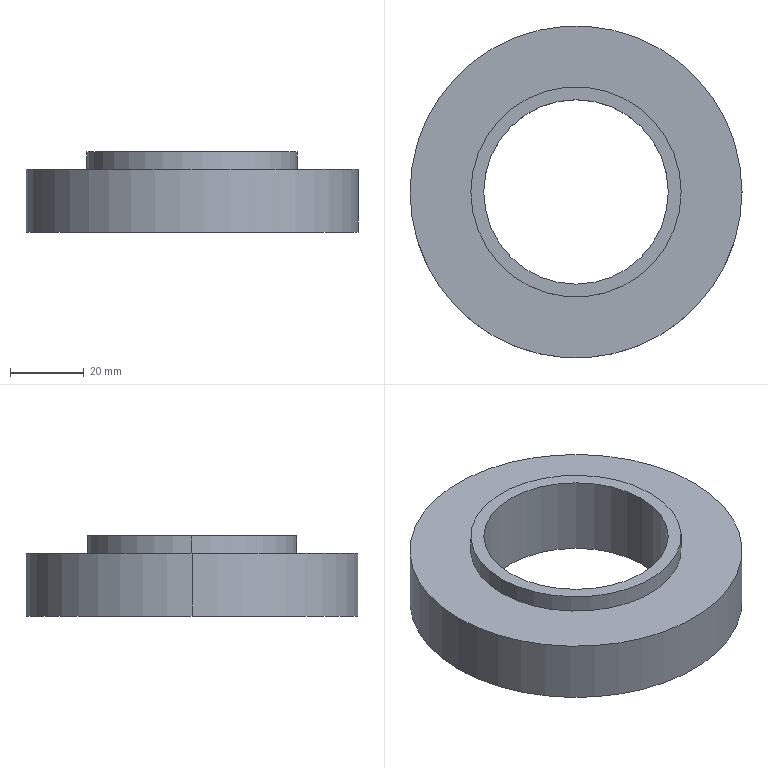Part | STEP file | 30210 | 1 solid | 9 faces | box 90 x 90 x 21.75 mm | volume 77564 mm3 | cylinder 6 | plane 3 | commonest cylinder face diameters 50 x2 57 x2 90 x2
STEP:
#1=CARTESIAN_POINT('',(0.,0.,0.));
#2=DIRECTION('',(0.,0.,1.));
#3=DIRECTION('',(1.,0.,0.));
#4=AXIS2_PLACEMENT_3D('',#1,#2,#3);
#5=CARTESIAN_POINT('',(-25.,0.,21.75));
#6=VERTEX_POINT('',#5);
#7=CARTESIAN_POINT('',(-25.,0.,0.));
#8=VERTEX_POINT('',#7);
#9=CARTESIAN_POINT('',(-25.,0.,21.75));
#10=DIRECTION('',(0.,0.,-1.));
#11=VECTOR('',#10,1.);
#12=LINE('',#9,#11);
#13=CARTESIAN_POINT('',(0.,0.,21.75));
#14=DIRECTION('',(0.,0.,-1.));
#15=DIRECTION('',(-1.,0.,0.));
#16=AXIS2_PLACEMENT_3D('',#13,#14,#15);
#17=CYLINDRICAL_SURFACE('',#16,25.);
#18=CARTESIAN_POINT('',(6.283,0.));
#19=DIRECTION('',(0.,1.));
#20=VECTOR('',#19,1.);
#21=LINE('',#18,#20);
#22=(GEOMETRIC_REPRESENTATION_CONTEXT(2)PARAMETRIC_REPRESENTATION_CONTEXT()REPRESENTATION_CONTEXT('',''));
#23=DEFINITIONAL_REPRESENTATION('',(#21),#22);
#24=PCURVE('',#17,#23);
#25=CARTESIAN_POINT('',(0.,0.,21.75));
#26=DIRECTION('',(0.,0.,-1.));
#27=DIRECTION('',(-1.,0.,0.));
#28=AXIS2_PLACEMENT_3D('',#25,#26,#27);
#29=CYLINDRICAL_SURFACE('',#28,25.);
#30=CARTESIAN_POINT('',(0.,0.));
#31=DIRECTION('',(0.,1.));
#32=VECTOR('',#31,1.);
#33=LINE('',#30,#32);
#34=(GEOMETRIC_REPRESENTATION_CONTEXT(2)PARAMETRIC_REPRESENTATION_CONTEXT()REPRESENTATION_CONTEXT('',''));
#35=DEFINITIONAL_REPRESENTATION('',(#33),#34);
#36=PCURVE('',#29,#35);
#37=SURFACE_CURVE('',#12,(#24,#36),.PCURVE_S1.);
#38=EDGE_CURVE('',#6,#8,#37,.T.);
#39=ORIENTED_EDGE('',*,*,#38,.T.);
#40=CARTESIAN_POINT('',(25.,0.,0.));
#41=VERTEX_POINT('',#40);
#42=CARTESIAN_POINT('',(0.,0.,0.));
#43=DIRECTION('',(0.,0.,-1.));
#44=DIRECTION('',(-1.,0.,0.));
#45=AXIS2_PLACEMENT_3D('',#42,#43,#44);
#46=CIRCLE('',#45,25.);
#47=CARTESIAN_POINT('',(0.,21.75));
#48=DIRECTION('',(1.,0.));
#49=VECTOR('',#48,1.);
#50=LINE('',#47,#49);
#51=(GEOMETRIC_REPRESENTATION_CONTEXT(2)PARAMETRIC_REPRESENTATION_CONTEXT()REPRESENTATION_CONTEXT('',''));
#52=DEFINITIONAL_REPRESENTATION('',(#50),#51);
#53=PCURVE('',#17,#52);
#54=CARTESIAN_POINT('',(0.,0.,0.));
#55=DIRECTION('',(0.,0.,1.));
#56=DIRECTION('',(1.,0.,0.));
#57=AXIS2_PLACEMENT_3D('',#54,#55,#56);
#58=PLANE('',#57);
#59=CARTESIAN_POINT('',(-25.,0.));
#60=CARTESIAN_POINT('',(-25.,43.301));
#61=CARTESIAN_POINT('',(12.5,21.651));
#62=CARTESIAN_POINT('',(50.,0.));
#63=CARTESIAN_POINT('',(12.5,-21.651));
#64=CARTESIAN_POINT('',(-25.,-43.301));
#65=CARTESIAN_POINT('',(-25.,0.));
#66=(BOUNDED_CURVE()B_SPLINE_CURVE(2,(#59,#60,#61,#62,#63,#64,#65),.UNSPECIFIED.,.T.,.F.)B_SPLINE_CURVE_WITH_KNOTS((1,2,2,2,2,1),(-2.094,0.,2.094,4.189,6.283,8.378),.UNSPECIFIED.)CURVE()GEOMETRIC_REPRESENTATION_ITEM()RATIONAL_B_SPLINE_CURVE((1.,0.5,1.,0.5,1.,0.5,1.))REPRESENTATION_ITEM(''));
#67=(GEOMETRIC_REPRESENTATION_CONTEXT(2)PARAMETRIC_REPRESENTATION_CONTEXT()REPRESENTATION_CONTEXT('',''));
#68=DEFINITIONAL_REPRESENTATION('',(#66),#67);
#69=PCURVE('',#58,#68);
#70=SURFACE_CURVE('',#46,(#53,#69),.PCURVE_S1.);
#71=EDGE_CURVE('',#41,#8,#70,.T.);
#72=ORIENTED_EDGE('',*,*,#71,.F.);
#73=CARTESIAN_POINT('',(25.,0.,21.75));
#74=VERTEX_POINT('',#73);
#75=CARTESIAN_POINT('',(25.,0.,21.75));
#76=DIRECTION('',(0.,0.,-1.));
#77=VECTOR('',#76,1.);
#78=LINE('',#75,#77);
#79=CARTESIAN_POINT('',(3.142,0.));
#80=DIRECTION('',(0.,1.));
#81=VECTOR('',#80,1.);
#82=LINE('',#79,#81);
#83=(GEOMETRIC_REPRESENTATION_CONTEXT(2)PARAMETRIC_REPRESENTATION_CONTEXT()REPRESENTATION_CONTEXT('',''));
#84=DEFINITIONAL_REPRESENTATION('',(#82),#83);
#85=PCURVE('',#17,#84);
#86=CARTESIAN_POINT('',(3.142,0.));
#87=DIRECTION('',(0.,1.));
#88=VECTOR('',#87,1.);
#89=LINE('',#86,#88);
#90=(GEOMETRIC_REPRESENTATION_CONTEXT(2)PARAMETRIC_REPRESENTATION_CONTEXT()REPRESENTATION_CONTEXT('',''));
#91=DEFINITIONAL_REPRESENTATION('',(#89),#90);
#92=PCURVE('',#29,#91);
#93=SURFACE_CURVE('',#78,(#85,#92),.PCURVE_S1.);
#94=EDGE_CURVE('',#74,#41,#93,.T.);
#95=ORIENTED_EDGE('',*,*,#94,.F.);
#96=CARTESIAN_POINT('',(0.,0.,21.75));
#97=DIRECTION('',(0.,0.,-1.));
#98=DIRECTION('',(-1.,0.,0.));
#99=AXIS2_PLACEMENT_3D('',#96,#97,#98);
#100=CIRCLE('',#99,25.);
#101=CARTESIAN_POINT('',(0.,0.));
#102=DIRECTION('',(1.,0.));
#103=VECTOR('',#102,1.);
#104=LINE('',#101,#103);
#105=(GEOMETRIC_REPRESENTATION_CONTEXT(2)PARAMETRIC_REPRESENTATION_CONTEXT()REPRESENTATION_CONTEXT('',''));
#106=DEFINITIONAL_REPRESENTATION('',(#104),#105);
#107=PCURVE('',#17,#106);
#108=CARTESIAN_POINT('',(0.,0.,21.75));
#109=DIRECTION('',(0.,0.,1.));
#110=DIRECTION('',(1.,0.,0.));
#111=AXIS2_PLACEMENT_3D('',#108,#109,#110);
#112=PLANE('',#111);
#113=CARTESIAN_POINT('',(-25.,0.));
#114=CARTESIAN_POINT('',(-25.,43.301));
#115=CARTESIAN_POINT('',(12.5,21.651));
#116=CARTESIAN_POINT('',(50.,0.));
#117=CARTESIAN_POINT('',(12.5,-21.651));
#118=CARTESIAN_POINT('',(-25.,-43.301));
#119=CARTESIAN_POINT('',(-25.,0.));
#120=(BOUNDED_CURVE()B_SPLINE_CURVE(2,(#113,#114,#115,#116,#117,#118,#119),.UNSPECIFIED.,.T.,.F.)B_SPLINE_CURVE_WITH_KNOTS((1,2,2,2,2,1),(-2.094,0.,2.094,4.189,6.283,8.378),.UNSPECIFIED.)CURVE()GEOMETRIC_REPRESENTATION_ITEM()RATIONAL_B_SPLINE_CURVE((1.,0.5,1.,0.5,1.,0.5,1.))REPRESENTATION_ITEM(''));
#121=(GEOMETRIC_REPRESENTATION_CONTEXT(2)PARAMETRIC_REPRESENTATION_CONTEXT()REPRESENTATION_CONTEXT('',''));
#122=DEFINITIONAL_REPRESENTATION('',(#120),#121);
#123=PCURVE('',#112,#122);
#124=SURFACE_CURVE('',#100,(#107,#123),.PCURVE_S1.);
#125=EDGE_CURVE('',#74,#6,#124,.T.);
#126=ORIENTED_EDGE('',*,*,#125,.T.);
#127=EDGE_LOOP('',(#39,#72,#95,#126));
#128=FACE_BOUND('',#127,.F.);
#129=ADVANCED_FACE('',(#128),#17,.F.);
#130=CARTESIAN_POINT('',(-45.,0.,17.));
#131=VERTEX_POINT('',#130);
#132=CARTESIAN_POINT('',(45.,0.,17.));
#133=VERTEX_POINT('',#132);
#134=CARTESIAN_POINT('',(0.,0.,17.));
#135=DIRECTION('',(0.,0.,-1.));
#136=DIRECTION('',(-1.,0.,0.));
#137=AXIS2_PLACEMENT_3D('',#134,#135,#136);
#138=CIRCLE('',#137,45.);
#139=CARTESIAN_POINT('',(0.,0.,21.75));
#140=DIRECTION('',(0.,0.,-1.));
#141=DIRECTION('',(-1.,0.,0.));
#142=AXIS2_PLACEMENT_3D('',#139,#140,#141);
#143=CYLINDRICAL_SURFACE('',#142,45.);
#144=CARTESIAN_POINT('',(0.,4.75));
#145=DIRECTION('',(1.,0.));
#146=VECTOR('',#145,1.);
#147=LINE('',#144,#146);
#148=(GEOMETRIC_REPRESENTATION_CONTEXT(2)PARAMETRIC_REPRESENTATION_CONTEXT()REPRESENTATION_CONTEXT('',''));
#149=DEFINITIONAL_REPRESENTATION('',(#147),#148);
#150=PCURVE('',#143,#149);
#151=CARTESIAN_POINT('',(0.,0.,17.));
#152=DIRECTION('',(0.,0.,1.));
#153=DIRECTION('',(1.,0.,0.));
#154=AXIS2_PLACEMENT_3D('',#151,#152,#153);
#155=PLANE('',#154);
#156=CARTESIAN_POINT('',(-45.,0.));
#157=CARTESIAN_POINT('',(-45.,77.942));
#158=CARTESIAN_POINT('',(22.5,38.971));
#159=CARTESIAN_POINT('',(90.,0.));
#160=CARTESIAN_POINT('',(22.5,-38.971));
#161=CARTESIAN_POINT('',(-45.,-77.942));
#162=CARTESIAN_POINT('',(-45.,0.));
#163=(BOUNDED_CURVE()B_SPLINE_CURVE(2,(#156,#157,#158,#159,#160,#161,#162),.UNSPECIFIED.,.T.,.F.)B_SPLINE_CURVE_WITH_KNOTS((1,2,2,2,2,1),(-2.094,0.,2.094,4.189,6.283,8.378),.UNSPECIFIED.)CURVE()GEOMETRIC_REPRESENTATION_ITEM()RATIONAL_B_SPLINE_CURVE((1.,0.5,1.,0.5,1.,0.5,1.))REPRESENTATION_ITEM(''));
#164=(GEOMETRIC_REPRESENTATION_CONTEXT(2)PARAMETRIC_REPRESENTATION_CONTEXT()REPRESENTATION_CONTEXT('',''));
#165=DEFINITIONAL_REPRESENTATION('',(#163),#164);
#166=PCURVE('',#155,#165);
#167=SURFACE_CURVE('',#138,(#150,#166),.PCURVE_S1.);
#168=EDGE_CURVE('',#131,#133,#167,.T.);
#169=ORIENTED_EDGE('',*,*,#168,.T.);
#170=CARTESIAN_POINT('',(45.,0.,0.));
#171=VERTEX_POINT('',#170);
#172=CARTESIAN_POINT('',(45.,0.,21.75));
#173=DIRECTION('',(0.,0.,-1.));
#174=VECTOR('',#173,1.);
#175=LINE('',#172,#174);
#176=CARTESIAN_POINT('',(3.142,0.));
#177=DIRECTION('',(0.,1.));
#178=VECTOR('',#177,1.);
#179=LINE('',#176,#178);
#180=(GEOMETRIC_REPRESENTATION_CONTEXT(2)PARAMETRIC_REPRESENTATION_CONTEXT()REPRESENTATION_CONTEXT('',''));
#181=DEFINITIONAL_REPRESENTATION('',(#179),#180);
#182=PCURVE('',#143,#181);
#183=CARTESIAN_POINT('',(0.,0.,21.75));
#184=DIRECTION('',(0.,0.,-1.));
#185=DIRECTION('',(-1.,0.,0.));
#186=AXIS2_PLACEMENT_3D('',#183,#184,#185);
#187=CYLINDRICAL_SURFACE('',#186,45.);
#188=CARTESIAN_POINT('',(3.142,0.));
#189=DIRECTION('',(0.,1.));
#190=VECTOR('',#189,1.);
#191=LINE('',#188,#190);
#192=(GEOMETRIC_REPRESENTATION_CONTEXT(2)PARAMETRIC_REPRESENTATION_CONTEXT()REPRESENTATION_CONTEXT('',''));
#193=DEFINITIONAL_REPRESENTATION('',(#191),#192);
#194=PCURVE('',#187,#193);
#195=SURFACE_CURVE('',#175,(#182,#194),.PCURVE_S1.);
#196=EDGE_CURVE('',#133,#171,#195,.T.);
#197=ORIENTED_EDGE('',*,*,#196,.T.);
#198=CARTESIAN_POINT('',(-45.,0.,0.));
#199=VERTEX_POINT('',#198);
#200=CARTESIAN_POINT('',(0.,0.,0.));
#201=DIRECTION('',(0.,0.,1.));
#202=DIRECTION('',(-1.,0.,0.));
#203=AXIS2_PLACEMENT_3D('',#200,#201,#202);
#204=CIRCLE('',#203,45.);
#205=CARTESIAN_POINT('',(6.283,21.75));
#206=DIRECTION('',(-1.,0.));
#207=VECTOR('',#206,1.);
#208=LINE('',#205,#207);
#209=(GEOMETRIC_REPRESENTATION_CONTEXT(2)PARAMETRIC_REPRESENTATION_CONTEXT()REPRESENTATION_CONTEXT('',''));
#210=DEFINITIONAL_REPRESENTATION('',(#208),#209);
#211=PCURVE('',#143,#210);
#212=CARTESIAN_POINT('',(0.,0.));
#213=DIRECTION('',(-1.,0.));
#214=AXIS2_PLACEMENT_2D('',#212,#213);
#215=CIRCLE('',#214,45.);
#216=(GEOMETRIC_REPRESENTATION_CONTEXT(2)PARAMETRIC_REPRESENTATION_CONTEXT()REPRESENTATION_CONTEXT('',''));
#217=DEFINITIONAL_REPRESENTATION('',(#215),#216);
#218=PCURVE('',#58,#217);
#219=SURFACE_CURVE('',#204,(#211,#218),.PCURVE_S1.);
#220=EDGE_CURVE('',#171,#199,#219,.T.);
#221=ORIENTED_EDGE('',*,*,#220,.T.);
#222=CARTESIAN_POINT('',(-45.,0.,21.75));
#223=DIRECTION('',(0.,0.,-1.));
#224=VECTOR('',#223,1.);
#225=LINE('',#222,#224);
#226=CARTESIAN_POINT('',(0.,0.));
#227=DIRECTION('',(0.,1.));
#228=VECTOR('',#227,1.);
#229=LINE('',#226,#228);
#230=(GEOMETRIC_REPRESENTATION_CONTEXT(2)PARAMETRIC_REPRESENTATION_CONTEXT()REPRESENTATION_CONTEXT('',''));
#231=DEFINITIONAL_REPRESENTATION('',(#229),#230);
#232=PCURVE('',#143,#231);
#233=CARTESIAN_POINT('',(6.283,0.));
#234=DIRECTION('',(0.,1.));
#235=VECTOR('',#234,1.);
#236=LINE('',#233,#235);
#237=(GEOMETRIC_REPRESENTATION_CONTEXT(2)PARAMETRIC_REPRESENTATION_CONTEXT()REPRESENTATION_CONTEXT('',''));
#238=DEFINITIONAL_REPRESENTATION('',(#236),#237);
#239=PCURVE('',#187,#238);
#240=SURFACE_CURVE('',#225,(#232,#239),.PCURVE_S1.);
#241=EDGE_CURVE('',#131,#199,#240,.T.);
#242=ORIENTED_EDGE('',*,*,#241,.F.);
#243=EDGE_LOOP('',(#169,#197,#221,#242));
#244=FACE_BOUND('',#243,.T.);
#245=ADVANCED_FACE('',(#244),#143,.T.);
#246=CARTESIAN_POINT('',(-28.5,0.,17.));
#247=VERTEX_POINT('',#246);
#248=CARTESIAN_POINT('',(28.5,0.,17.));
#249=VERTEX_POINT('',#248);
#250=CARTESIAN_POINT('',(0.,0.,17.));
#251=DIRECTION('',(0.,0.,-1.));
#252=DIRECTION('',(1.,0.,0.));
#253=AXIS2_PLACEMENT_3D('',#250,#251,#252);
#254=CIRCLE('',#253,28.5);
#255=CARTESIAN_POINT('',(0.,0.,17.));
#256=DIRECTION('',(0.,0.,1.));
#257=DIRECTION('',(1.,0.,0.));
#258=AXIS2_PLACEMENT_3D('',#255,#256,#257);
#259=CYLINDRICAL_SURFACE('',#258,28.5);
#260=CARTESIAN_POINT('',(6.283,0.));
#261=DIRECTION('',(-1.,0.));
#262=VECTOR('',#261,1.);
#263=LINE('',#260,#262);
#264=(GEOMETRIC_REPRESENTATION_CONTEXT(2)PARAMETRIC_REPRESENTATION_CONTEXT()REPRESENTATION_CONTEXT('',''));
#265=DEFINITIONAL_REPRESENTATION('',(#263),#264);
#266=PCURVE('',#259,#265);
#267=CARTESIAN_POINT('',(28.5,0.));
#268=CARTESIAN_POINT('',(28.5,-49.363));
#269=CARTESIAN_POINT('',(-14.25,-24.682));
#270=CARTESIAN_POINT('',(-57.,0.));
#271=CARTESIAN_POINT('',(-14.25,24.682));
#272=CARTESIAN_POINT('',(28.5,49.363));
#273=CARTESIAN_POINT('',(28.5,0.));
#274=(BOUNDED_CURVE()B_SPLINE_CURVE(2,(#267,#268,#269,#270,#271,#272,#273),.UNSPECIFIED.,.T.,.F.)B_SPLINE_CURVE_WITH_KNOTS((1,2,2,2,2,1),(-2.094,0.,2.094,4.189,6.283,8.378),.UNSPECIFIED.)CURVE()GEOMETRIC_REPRESENTATION_ITEM()RATIONAL_B_SPLINE_CURVE((1.,0.5,1.,0.5,1.,0.5,1.))REPRESENTATION_ITEM(''));
#275=(GEOMETRIC_REPRESENTATION_CONTEXT(2)PARAMETRIC_REPRESENTATION_CONTEXT()REPRESENTATION_CONTEXT('',''));
#276=DEFINITIONAL_REPRESENTATION('',(#274),#275);
#277=PCURVE('',#155,#276);
#278=SURFACE_CURVE('',#254,(#266,#277),.PCURVE_S1.);
#279=EDGE_CURVE('',#247,#249,#278,.T.);
#280=ORIENTED_EDGE('',*,*,#279,.F.);
#281=CARTESIAN_POINT('',(-28.5,0.,21.75));
#282=VERTEX_POINT('',#281);
#283=CARTESIAN_POINT('',(-28.5,0.,17.));
#284=DIRECTION('',(0.,0.,1.));
#285=VECTOR('',#284,1.);
#286=LINE('',#283,#285);
#287=CARTESIAN_POINT('',(3.142,0.));
#288=DIRECTION('',(0.,1.));
#289=VECTOR('',#288,1.);
#290=LINE('',#287,#289);
#291=(GEOMETRIC_REPRESENTATION_CONTEXT(2)PARAMETRIC_REPRESENTATION_CONTEXT()REPRESENTATION_CONTEXT('',''));
#292=DEFINITIONAL_REPRESENTATION('',(#290),#291);
#293=PCURVE('',#259,#292);
#294=CARTESIAN_POINT('',(0.,0.,17.));
#295=DIRECTION('',(0.,0.,1.));
#296=DIRECTION('',(1.,0.,0.));
#297=AXIS2_PLACEMENT_3D('',#294,#295,#296);
#298=CYLINDRICAL_SURFACE('',#297,28.5);
#299=CARTESIAN_POINT('',(3.142,0.));
#300=DIRECTION('',(0.,1.));
#301=VECTOR('',#300,1.);
#302=LINE('',#299,#301);
#303=(GEOMETRIC_REPRESENTATION_CONTEXT(2)PARAMETRIC_REPRESENTATION_CONTEXT()REPRESENTATION_CONTEXT('',''));
#304=DEFINITIONAL_REPRESENTATION('',(#302),#303);
#305=PCURVE('',#298,#304);
#306=SURFACE_CURVE('',#286,(#293,#305),.PCURVE_S1.);
#307=EDGE_CURVE('',#247,#282,#306,.T.);
#308=ORIENTED_EDGE('',*,*,#307,.T.);
#309=CARTESIAN_POINT('',(28.5,0.,21.75));
#310=VERTEX_POINT('',#309);
#311=CARTESIAN_POINT('',(0.,0.,21.75));
#312=DIRECTION('',(0.,0.,1.));
#313=DIRECTION('',(1.,0.,0.));
#314=AXIS2_PLACEMENT_3D('',#311,#312,#313);
#315=CIRCLE('',#314,28.5);
#316=CARTESIAN_POINT('',(0.,4.75));
#317=DIRECTION('',(1.,0.));
#318=VECTOR('',#317,1.);
#319=LINE('',#316,#318);
#320=(GEOMETRIC_REPRESENTATION_CONTEXT(2)PARAMETRIC_REPRESENTATION_CONTEXT()REPRESENTATION_CONTEXT('',''));
#321=DEFINITIONAL_REPRESENTATION('',(#319),#320);
#322=PCURVE('',#259,#321);
#323=CARTESIAN_POINT('',(0.,0.));
#324=DIRECTION('',(1.,0.));
#325=AXIS2_PLACEMENT_2D('',#323,#324);
#326=CIRCLE('',#325,28.5);
#327=(GEOMETRIC_REPRESENTATION_CONTEXT(2)PARAMETRIC_REPRESENTATION_CONTEXT()REPRESENTATION_CONTEXT('',''));
#328=DEFINITIONAL_REPRESENTATION('',(#326),#327);
#329=PCURVE('',#112,#328);
#330=SURFACE_CURVE('',#315,(#322,#329),.PCURVE_S1.);
#331=EDGE_CURVE('',#310,#282,#330,.T.);
#332=ORIENTED_EDGE('',*,*,#331,.F.);
#333=CARTESIAN_POINT('',(28.5,0.,17.));
#334=DIRECTION('',(0.,0.,1.));
#335=VECTOR('',#334,1.);
#336=LINE('',#333,#335);
#337=CARTESIAN_POINT('',(0.,0.));
#338=DIRECTION('',(0.,1.));
#339=VECTOR('',#338,1.);
#340=LINE('',#337,#339);
#341=(GEOMETRIC_REPRESENTATION_CONTEXT(2)PARAMETRIC_REPRESENTATION_CONTEXT()REPRESENTATION_CONTEXT('',''));
#342=DEFINITIONAL_REPRESENTATION('',(#340),#341);
#343=PCURVE('',#259,#342);
#344=CARTESIAN_POINT('',(6.283,0.));
#345=DIRECTION('',(0.,1.));
#346=VECTOR('',#345,1.);
#347=LINE('',#344,#346);
#348=(GEOMETRIC_REPRESENTATION_CONTEXT(2)PARAMETRIC_REPRESENTATION_CONTEXT()REPRESENTATION_CONTEXT('',''));
#349=DEFINITIONAL_REPRESENTATION('',(#347),#348);
#350=PCURVE('',#298,#349);
#351=SURFACE_CURVE('',#336,(#343,#350),.PCURVE_S1.);
#352=EDGE_CURVE('',#249,#310,#351,.T.);
#353=ORIENTED_EDGE('',*,*,#352,.F.);
#354=EDGE_LOOP('',(#280,#308,#332,#353));
#355=FACE_BOUND('',#354,.T.);
#356=ADVANCED_FACE('',(#355),#259,.T.);
#357=CARTESIAN_POINT('',(0.,0.,0.));
#358=DIRECTION('',(0.,0.,-1.));
#359=DIRECTION('',(-1.,0.,0.));
#360=AXIS2_PLACEMENT_3D('',#357,#358,#359);
#361=CIRCLE('',#360,25.);
#362=CARTESIAN_POINT('',(-25.,0.));
#363=CARTESIAN_POINT('',(-25.,43.301));
#364=CARTESIAN_POINT('',(12.5,21.651));
#365=CARTESIAN_POINT('',(50.,0.));
#366=CARTESIAN_POINT('',(12.5,-21.651));
#367=CARTESIAN_POINT('',(-25.,-43.301));
#368=CARTESIAN_POINT('',(-25.,0.));
#369=(BOUNDED_CURVE()B_SPLINE_CURVE(2,(#362,#363,#364,#365,#366,#367,#368),.UNSPECIFIED.,.T.,.F.)B_SPLINE_CURVE_WITH_KNOTS((1,2,2,2,2,1),(-2.094,0.,2.094,4.189,6.283,8.378),.UNSPECIFIED.)CURVE()GEOMETRIC_REPRESENTATION_ITEM()RATIONAL_B_SPLINE_CURVE((1.,0.5,1.,0.5,1.,0.5,1.))REPRESENTATION_ITEM(''));
#370=(GEOMETRIC_REPRESENTATION_CONTEXT(2)PARAMETRIC_REPRESENTATION_CONTEXT()REPRESENTATION_CONTEXT('',''));
#371=DEFINITIONAL_REPRESENTATION('',(#369),#370);
#372=PCURVE('',#58,#371);
#373=CARTESIAN_POINT('',(0.,21.75));
#374=DIRECTION('',(1.,0.));
#375=VECTOR('',#374,1.);
#376=LINE('',#373,#375);
#377=(GEOMETRIC_REPRESENTATION_CONTEXT(2)PARAMETRIC_REPRESENTATION_CONTEXT()REPRESENTATION_CONTEXT('',''));
#378=DEFINITIONAL_REPRESENTATION('',(#376),#377);
#379=PCURVE('',#29,#378);
#380=SURFACE_CURVE('',#361,(#372,#379),.PCURVE_S1.);
#381=EDGE_CURVE('',#8,#41,#380,.T.);
#382=ORIENTED_EDGE('',*,*,#381,.F.);
#383=ORIENTED_EDGE('',*,*,#71,.F.);
#384=EDGE_LOOP('',(#382,#383));
#385=FACE_BOUND('',#384,.T.);
#386=CARTESIAN_POINT('',(0.,0.,0.));
#387=DIRECTION('',(0.,0.,1.));
#388=DIRECTION('',(-1.,0.,0.));
#389=AXIS2_PLACEMENT_3D('',#386,#387,#388);
#390=CIRCLE('',#389,45.);
#391=CARTESIAN_POINT('',(0.,0.));
#392=DIRECTION('',(-1.,0.));
#393=AXIS2_PLACEMENT_2D('',#391,#392);
#394=CIRCLE('',#393,45.);
#395=(GEOMETRIC_REPRESENTATION_CONTEXT(2)PARAMETRIC_REPRESENTATION_CONTEXT()REPRESENTATION_CONTEXT('',''));
#396=DEFINITIONAL_REPRESENTATION('',(#394),#395);
#397=PCURVE('',#58,#396);
#398=CARTESIAN_POINT('',(6.283,21.75));
#399=DIRECTION('',(-1.,0.));
#400=VECTOR('',#399,1.);
#401=LINE('',#398,#400);
#402=(GEOMETRIC_REPRESENTATION_CONTEXT(2)PARAMETRIC_REPRESENTATION_CONTEXT()REPRESENTATION_CONTEXT('',''));
#403=DEFINITIONAL_REPRESENTATION('',(#401),#402);
#404=PCURVE('',#187,#403);
#405=SURFACE_CURVE('',#390,(#397,#404),.PCURVE_S1.);
#406=EDGE_CURVE('',#199,#171,#405,.T.);
#407=ORIENTED_EDGE('',*,*,#406,.F.);
#408=ORIENTED_EDGE('',*,*,#220,.F.);
#409=EDGE_LOOP('',(#407,#408));
#410=FACE_BOUND('',#409,.T.);
#411=ADVANCED_FACE('',(#385,#410),#58,.F.);
#412=ORIENTED_EDGE('',*,*,#381,.F.);
#413=ORIENTED_EDGE('',*,*,#38,.F.);
#414=CARTESIAN_POINT('',(0.,0.,21.75));
#415=DIRECTION('',(0.,0.,-1.));
#416=DIRECTION('',(-1.,0.,0.));
#417=AXIS2_PLACEMENT_3D('',#414,#415,#416);
#418=CIRCLE('',#417,25.);
#419=CARTESIAN_POINT('',(0.,0.));
#420=DIRECTION('',(1.,0.));
#421=VECTOR('',#420,1.);
#422=LINE('',#419,#421);
#423=(GEOMETRIC_REPRESENTATION_CONTEXT(2)PARAMETRIC_REPRESENTATION_CONTEXT()REPRESENTATION_CONTEXT('',''));
#424=DEFINITIONAL_REPRESENTATION('',(#422),#423);
#425=PCURVE('',#29,#424);
#426=CARTESIAN_POINT('',(-25.,0.));
#427=CARTESIAN_POINT('',(-25.,43.301));
#428=CARTESIAN_POINT('',(12.5,21.651));
#429=CARTESIAN_POINT('',(50.,0.));
#430=CARTESIAN_POINT('',(12.5,-21.651));
#431=CARTESIAN_POINT('',(-25.,-43.301));
#432=CARTESIAN_POINT('',(-25.,0.));
#433=(BOUNDED_CURVE()B_SPLINE_CURVE(2,(#426,#427,#428,#429,#430,#431,#432),.UNSPECIFIED.,.T.,.F.)B_SPLINE_CURVE_WITH_KNOTS((1,2,2,2,2,1),(-2.094,0.,2.094,4.189,6.283,8.378),.UNSPECIFIED.)CURVE()GEOMETRIC_REPRESENTATION_ITEM()RATIONAL_B_SPLINE_CURVE((1.,0.5,1.,0.5,1.,0.5,1.))REPRESENTATION_ITEM(''));
#434=(GEOMETRIC_REPRESENTATION_CONTEXT(2)PARAMETRIC_REPRESENTATION_CONTEXT()REPRESENTATION_CONTEXT('',''));
#435=DEFINITIONAL_REPRESENTATION('',(#433),#434);
#436=PCURVE('',#112,#435);
#437=SURFACE_CURVE('',#418,(#425,#436),.PCURVE_S1.);
#438=EDGE_CURVE('',#6,#74,#437,.T.);
#439=ORIENTED_EDGE('',*,*,#438,.T.);
#440=ORIENTED_EDGE('',*,*,#94,.T.);
#441=EDGE_LOOP('',(#412,#413,#439,#440));
#442=FACE_BOUND('',#441,.F.);
#443=ADVANCED_FACE('',(#442),#29,.F.);
#444=ORIENTED_EDGE('',*,*,#196,.F.);
#445=CARTESIAN_POINT('',(0.,0.,17.));
#446=DIRECTION('',(0.,0.,-1.));
#447=DIRECTION('',(-1.,0.,0.));
#448=AXIS2_PLACEMENT_3D('',#445,#446,#447);
#449=CIRCLE('',#448,45.);
#450=CARTESIAN_POINT('',(0.,4.75));
#451=DIRECTION('',(1.,0.));
#452=VECTOR('',#451,1.);
#453=LINE('',#450,#452);
#454=(GEOMETRIC_REPRESENTATION_CONTEXT(2)PARAMETRIC_REPRESENTATION_CONTEXT()REPRESENTATION_CONTEXT('',''));
#455=DEFINITIONAL_REPRESENTATION('',(#453),#454);
#456=PCURVE('',#187,#455);
#457=CARTESIAN_POINT('',(-45.,0.));
#458=CARTESIAN_POINT('',(-45.,77.942));
#459=CARTESIAN_POINT('',(22.5,38.971));
#460=CARTESIAN_POINT('',(90.,0.));
#461=CARTESIAN_POINT('',(22.5,-38.971));
#462=CARTESIAN_POINT('',(-45.,-77.942));
#463=CARTESIAN_POINT('',(-45.,0.));
#464=(BOUNDED_CURVE()B_SPLINE_CURVE(2,(#457,#458,#459,#460,#461,#462,#463),.UNSPECIFIED.,.T.,.F.)B_SPLINE_CURVE_WITH_KNOTS((1,2,2,2,2,1),(-2.094,0.,2.094,4.189,6.283,8.378),.UNSPECIFIED.)CURVE()GEOMETRIC_REPRESENTATION_ITEM()RATIONAL_B_SPLINE_CURVE((1.,0.5,1.,0.5,1.,0.5,1.))REPRESENTATION_ITEM(''));
#465=(GEOMETRIC_REPRESENTATION_CONTEXT(2)PARAMETRIC_REPRESENTATION_CONTEXT()REPRESENTATION_CONTEXT('',''));
#466=DEFINITIONAL_REPRESENTATION('',(#464),#465);
#467=PCURVE('',#155,#466);
#468=SURFACE_CURVE('',#449,(#456,#467),.PCURVE_S1.);
#469=EDGE_CURVE('',#133,#131,#468,.T.);
#470=ORIENTED_EDGE('',*,*,#469,.T.);
#471=ORIENTED_EDGE('',*,*,#241,.T.);
#472=ORIENTED_EDGE('',*,*,#406,.T.);
#473=EDGE_LOOP('',(#444,#470,#471,#472));
#474=FACE_BOUND('',#473,.T.);
#475=ADVANCED_FACE('',(#474),#187,.T.);
#476=ORIENTED_EDGE('',*,*,#331,.T.);
#477=CARTESIAN_POINT('',(0.,0.,21.75));
#478=DIRECTION('',(0.,0.,1.));
#479=DIRECTION('',(1.,0.,0.));
#480=AXIS2_PLACEMENT_3D('',#477,#478,#479);
#481=CIRCLE('',#480,28.5);
#482=CARTESIAN_POINT('',(0.,0.));
#483=DIRECTION('',(1.,0.));
#484=AXIS2_PLACEMENT_2D('',#482,#483);
#485=CIRCLE('',#484,28.5);
#486=(GEOMETRIC_REPRESENTATION_CONTEXT(2)PARAMETRIC_REPRESENTATION_CONTEXT()REPRESENTATION_CONTEXT('',''));
#487=DEFINITIONAL_REPRESENTATION('',(#485),#486);
#488=PCURVE('',#112,#487);
#489=CARTESIAN_POINT('',(0.,4.75));
#490=DIRECTION('',(1.,0.));
#491=VECTOR('',#490,1.);
#492=LINE('',#489,#491);
#493=(GEOMETRIC_REPRESENTATION_CONTEXT(2)PARAMETRIC_REPRESENTATION_CONTEXT()REPRESENTATION_CONTEXT('',''));
#494=DEFINITIONAL_REPRESENTATION('',(#492),#493);
#495=PCURVE('',#298,#494);
#496=SURFACE_CURVE('',#481,(#488,#495),.PCURVE_S1.);
#497=EDGE_CURVE('',#282,#310,#496,.T.);
#498=ORIENTED_EDGE('',*,*,#497,.T.);
#499=EDGE_LOOP('',(#476,#498));
#500=FACE_BOUND('',#499,.T.);
#501=ORIENTED_EDGE('',*,*,#438,.T.);
#502=ORIENTED_EDGE('',*,*,#125,.T.);
#503=EDGE_LOOP('',(#501,#502));
#504=FACE_BOUND('',#503,.T.);
#505=ADVANCED_FACE('',(#500,#504),#112,.T.);
#506=ORIENTED_EDGE('',*,*,#168,.F.);
#507=ORIENTED_EDGE('',*,*,#469,.F.);
#508=EDGE_LOOP('',(#506,#507));
#509=FACE_BOUND('',#508,.T.);
#510=CARTESIAN_POINT('',(0.,0.,17.));
#511=DIRECTION('',(0.,0.,-1.));
#512=DIRECTION('',(1.,0.,0.));
#513=AXIS2_PLACEMENT_3D('',#510,#511,#512);
#514=CIRCLE('',#513,28.5);
#515=CARTESIAN_POINT('',(28.5,0.));
#516=CARTESIAN_POINT('',(28.5,-49.363));
#517=CARTESIAN_POINT('',(-14.25,-24.682));
#518=CARTESIAN_POINT('',(-57.,0.));
#519=CARTESIAN_POINT('',(-14.25,24.682));
#520=CARTESIAN_POINT('',(28.5,49.363));
#521=CARTESIAN_POINT('',(28.5,0.));
#522=(BOUNDED_CURVE()B_SPLINE_CURVE(2,(#515,#516,#517,#518,#519,#520,#521),.UNSPECIFIED.,.T.,.F.)B_SPLINE_CURVE_WITH_KNOTS((1,2,2,2,2,1),(-2.094,0.,2.094,4.189,6.283,8.378),.UNSPECIFIED.)CURVE()GEOMETRIC_REPRESENTATION_ITEM()RATIONAL_B_SPLINE_CURVE((1.,0.5,1.,0.5,1.,0.5,1.))REPRESENTATION_ITEM(''));
#523=(GEOMETRIC_REPRESENTATION_CONTEXT(2)PARAMETRIC_REPRESENTATION_CONTEXT()REPRESENTATION_CONTEXT('',''));
#524=DEFINITIONAL_REPRESENTATION('',(#522),#523);
#525=PCURVE('',#155,#524);
#526=CARTESIAN_POINT('',(6.283,0.));
#527=DIRECTION('',(-1.,0.));
#528=VECTOR('',#527,1.);
#529=LINE('',#526,#528);
#530=(GEOMETRIC_REPRESENTATION_CONTEXT(2)PARAMETRIC_REPRESENTATION_CONTEXT()REPRESENTATION_CONTEXT('',''));
#531=DEFINITIONAL_REPRESENTATION('',(#529),#530);
#532=PCURVE('',#298,#531);
#533=SURFACE_CURVE('',#514,(#525,#532),.PCURVE_S1.);
#534=EDGE_CURVE('',#249,#247,#533,.T.);
#535=ORIENTED_EDGE('',*,*,#534,.T.);
#536=ORIENTED_EDGE('',*,*,#279,.T.);
#537=EDGE_LOOP('',(#535,#536));
#538=FACE_BOUND('',#537,.T.);
#539=ADVANCED_FACE('',(#509,#538),#155,.T.);
#540=ORIENTED_EDGE('',*,*,#307,.F.);
#541=ORIENTED_EDGE('',*,*,#534,.F.);
#542=ORIENTED_EDGE('',*,*,#352,.T.);
#543=ORIENTED_EDGE('',*,*,#497,.F.);
#544=EDGE_LOOP('',(#540,#541,#542,#543));
#545=FACE_BOUND('',#544,.T.);
#546=ADVANCED_FACE('',(#545),#298,.T.);
#547=CLOSED_SHELL('',(#129,#245,#356,#411,#443,#475,#505,#539,#546));
#548=MANIFOLD_SOLID_BREP('',#547);
#549=(LENGTH_UNIT()NAMED_UNIT(*)SI_UNIT(.MILLI.,.METRE.));
#550=UNCERTAINTY_MEASURE_WITH_UNIT(LENGTH_MEASURE(0.0000001),#549,'','');
#551=(NAMED_UNIT(*)PLANE_ANGLE_UNIT()SI_UNIT($,.RADIAN.));
#552=(NAMED_UNIT(*)SI_UNIT($,.STERADIAN.)SOLID_ANGLE_UNIT());
#553=(GEOMETRIC_REPRESENTATION_CONTEXT(3)GLOBAL_UNCERTAINTY_ASSIGNED_CONTEXT((#550))GLOBAL_UNIT_ASSIGNED_CONTEXT((#549,#551,#552))REPRESENTATION_CONTEXT('',''));
#554=ADVANCED_BREP_SHAPE_REPRESENTATION('',(#4,#548),#553);